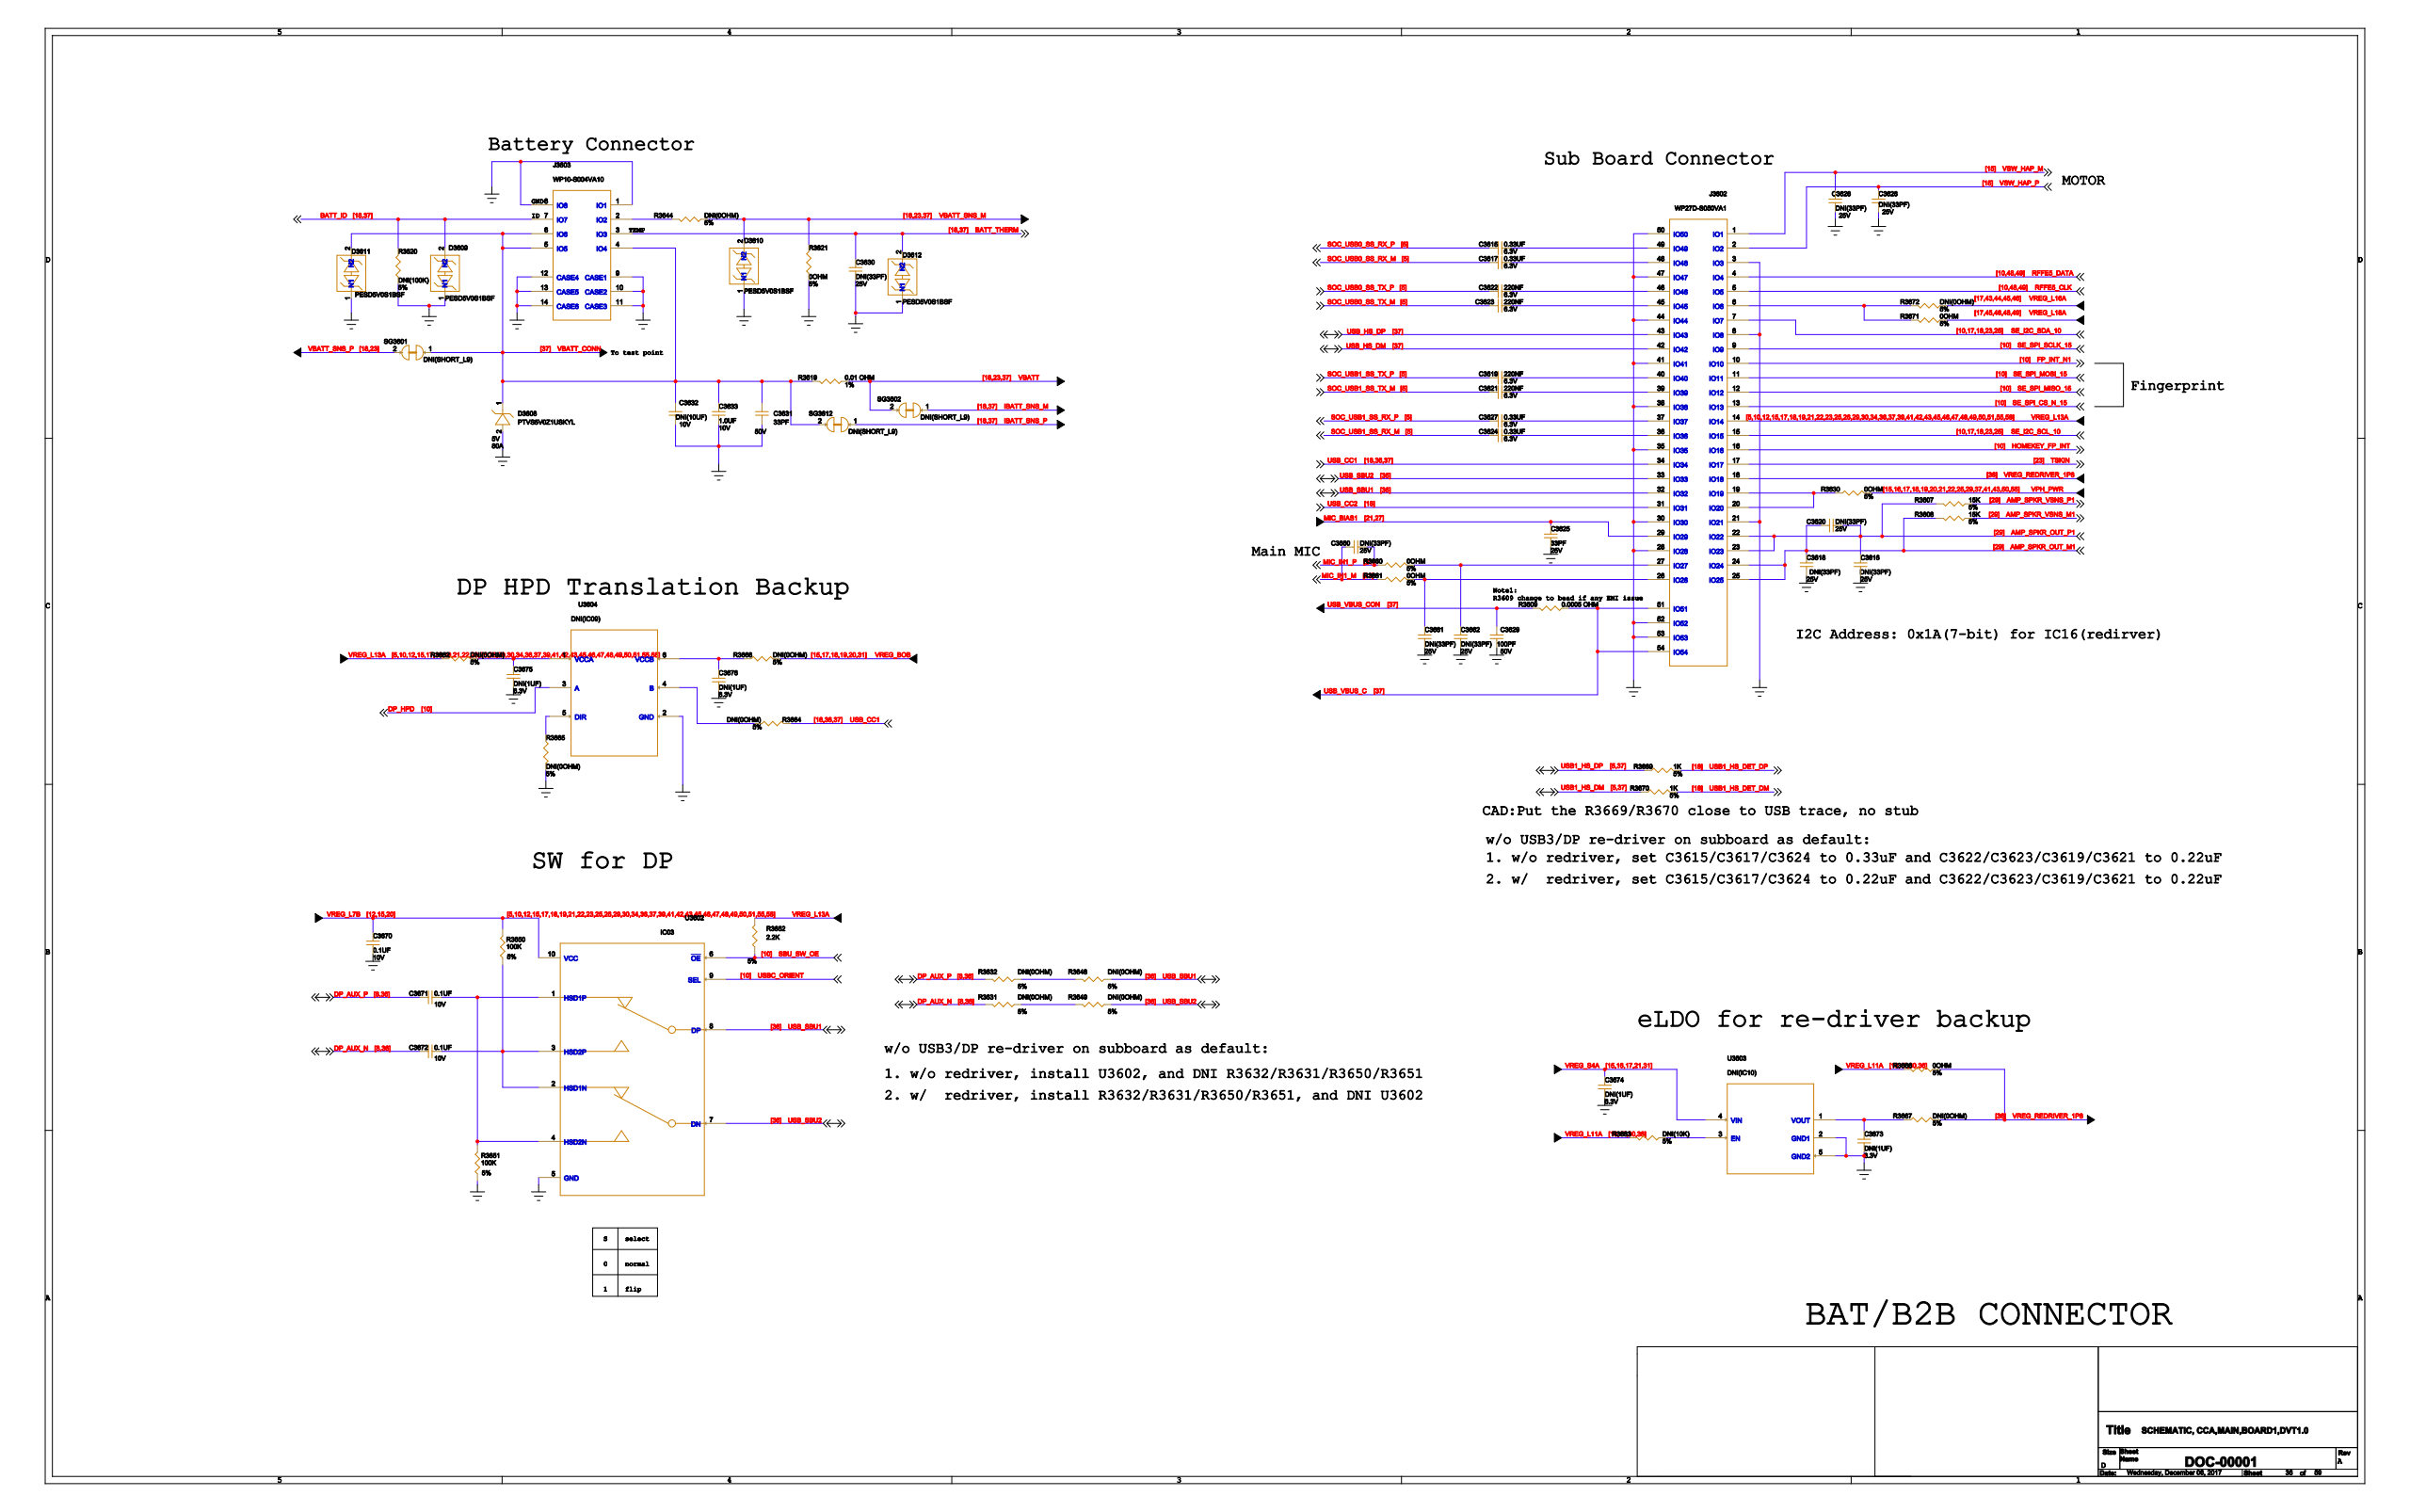Circuit board | KiCad | 1657 parts | 1365 nets | one sheet of the schematic
Parts on this sheet (reference | value | footprint):
C3615
C3616
C3617
C3618
C3619
C3620
C3621
C3622
C3623
C3624
C3625
C3626
C3627
C3628
C3629
C3630
C3631
C3632
C3633
C3660
C3661
C3662
C3670
C3671
C3672
C3673
C3674
C3675
C3676
D3608
D3609
D3610
D3611
D3612
J3602
J3603
R3607
R3608
R3609
R3619
R3620
R3621
R3630
R3631
R3632
R3644
R3648
R3649
R3650
R3651
R3652
R3660
R3661
R3662
R3663
R3664
R3665
R3666
R3667
R3668
R3669
R3670
R3671
R3672
SG3601
SG3602
SG3612
U3602
U3603
U3604
Nets of these parts (net: part-pin ...):
C_USB0_SS_RX_P: C3615-1
N46050206: C3615-2 J3602-49
GND: C3616-2 C3618-2 C3625-2 C3626-2 C3628-2 C3629-2 C3630-2 C3631-2 C3632-2 C3633-2 C3661-2 C3662-2 C3670-2 C3673-2 C3674-2 C3675-2 C3676-2 D3608-2 D3609-1 D3610-1 D3611-1 D3612-1 J3603-1 J3603-8 J3603-9 J3603-10 J3603-11 J3603-12 J3603-13 J3603-14 R3620-2 R3621-2 R3651-2 R3665-1 U3602-5 U3603-2 U3603-5 U3604-2 J3602-3 J3602-8 J3602-21 J3602-28 J3602-30 J3602-35 J3602-38 J3602-41 J3602-44 J3602-47 J3602-50 J3602-52 J3602-53
N21629163: C3662-1 R3660-2 J3602-27
VREG_L13A: R3652-1 R3662-2 J3602-14
VPH_PWR: R3630-2
VBATT_SNS_P: SG3601-2
N23465148: C3675-1 R3662-1 U3604-1
BATT_THERM: C3630-1 D3612-2 J3603-3
VSW_HAP_M: C3628-1 J3602-1
MP_SPKR_OUT_P1: C3616-1 C3620-2 R3607-2 J3602-22 J3602-23
MIC_BIAS1: C3625-1 J3602-29
USB_VBUS_CON: C3629-1 R3609-2
C_USB1_SS_RX_M: C3624-1
N46050432: C3624-2 J3602-36
TSKIN: J3602-17
G_REDRIVER_1P8: R3666-2 R3667-1 J3602-18
N23463313: C3673-1 R3667-2 U3603-1
USB1_HS_DET_DP: R3669-1
USB1_HS_DP: R3669-2
USB_HS_DP: J3602-43
USB_HS_DM: J3602-42
USB1_HS_DM: R3670-2
VREG_BOB: R3668-1
SE_I2C_SCL_10: J3602-15
SE_I2C_SDA_10: J3602-7
VREG_L11A: R3663-1 R3666-1
MIC_IN1_M: C3660-1 R3661-1
MIC_IN1_P: C3660-2 R3660-1
RFFE5_DATA: J3602-4
MP_SPKR_OUT_M1: C3618-1 C3620-1 R3608-2 J3602-24 J3602-25
N23466868: C3676-1 R3668-2 U3604-6
N21629180: C3661-1 R3661-2 J3602-26
C_USB1_SS_TX_M: C3621-1
N46050382: C3621-2 J3602-39
C_USB0_SS_TX_M: C3623-1
N46050244: C3623-2 J3602-45
VBATT_CONN: C3631-1 C3632-1 C3633-1 D3608-1 D3611-2 J3603-4 J3603-5 J3603-6 R3619-1 SG3601-1 SG3612-2
VBATT: R3619-2 SG3602-2
DP_AUX_P: C3671-1 R3632-1
N22306228: C3671-2 R3651-1 U3602-1 U3602-4
VREG_L7B: C3670-1 R3650-1 U3602-10
C_USB0_SS_RX_M: C3617-1
N46050167: C3617-2 J3602-48
DP_HPD: U3604-3
SBU_SW_OE: R3652-2 U3602-6
IBATT_SNS_M: SG3602-1
N22152425: R3671-1 R3672-1 J3602-6
VREG_L16A: R3672-2
DP_AUX_N: C3672-1 R3631-1
N23069335: R3631-2 R3649-1
VREG_L18A: R3671-2
P_SPKR_VSNS_M1: R3608-1
N23069308: R3632-2 R3648-1
N22306230: C3672-2 R3650-2 U3602-2 U3602-3
N23467179: R3664-1 U3604-4
USB_CC1: R3664-2 J3602-34
BATT_ID: D3609-2 J3603-7 R3620-1
N22128379: R3630-1 J3602-19 J3602-20
VREG_S4A: C3674-1 U3603-4
USB_SBU1: R3648-2 U3602-8 J3602-32
N23463264: R3663-2 U3603-3
N17001706: J3603-2 R3644-1
VBATT_SNS_M: D3610-2 R3621-1 R3644-2
N23465318: R3665-2 U3604-5
P_SPKR_VSNS_P1: R3607-1
VSW_HAP_P: C3626-1 J3602-2
C_USB1_SS_RX_P: C3627-1
N46049659: C3627-2 J3602-37
USB1_HS_DET_DM: R3670-1
USB_SBU2: R3649-2 U3602-7 J3602-33
RFFE5_CLK: J3602-5
C_USB0_SS_TX_P: C3622-1
USBC_ORIENT: U3602-9
C_USB1_SS_TX_P: C3619-1
SE_SPI_MISO_15: J3602-12
SE_SPI_MOSI_15: J3602-11
SE_SPI_SCLK_15: J3602-9
FP_INT_N1: J3602-10
SE_SPI_CS_N_15: J3602-13
HOMEKEY_FP_INT: J3602-16
IBATT_SNS_P: SG3612-1
N46049903: C3619-2 J3602-40
USB_VBUS_C: R3609-1 J3602-51 J3602-54
USB_CC2: J3602-31
N46050290: C3622-2 J3602-46